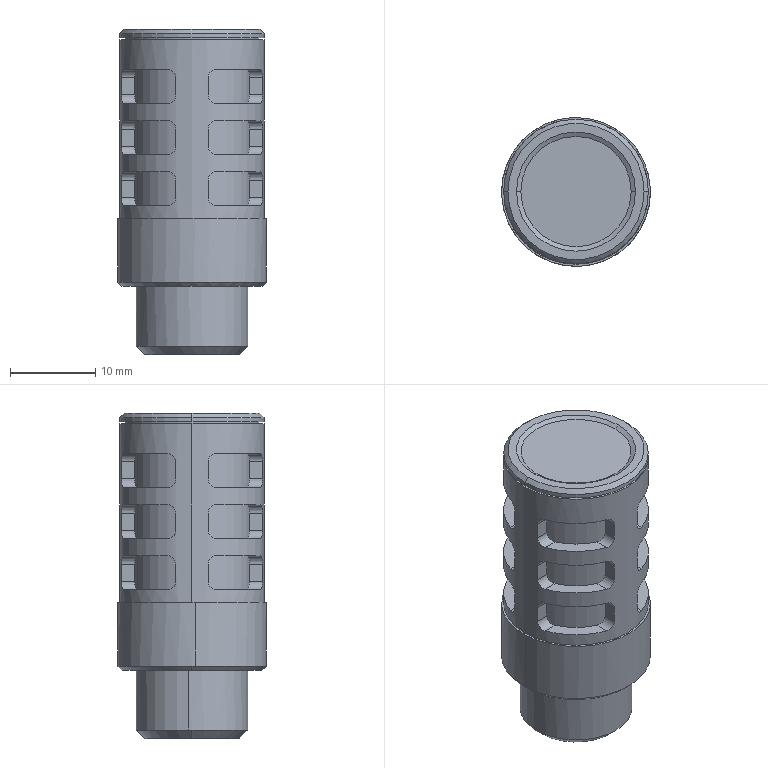Part | NX | 1 solid | 133 faces | box 17.5 x 17.5 x 38.2 mm | volume 7385 mm3 | cylinder 70 | plane 55 | cone 8 | commonest cylinder face diameters 2 x48 14 x12 17 x4 13.157 x2 15.8 x2 17.5 x2